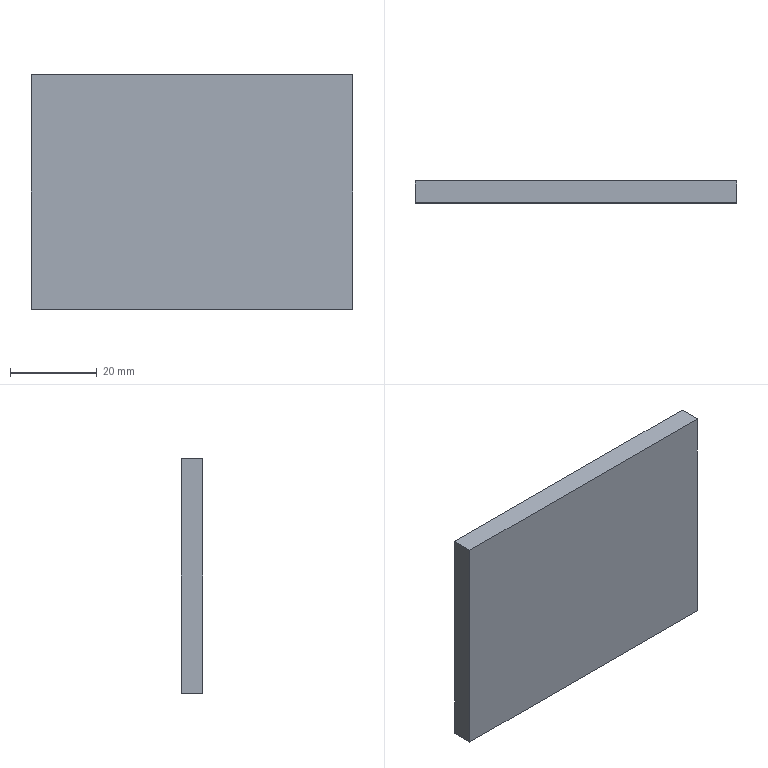Part | STEP file | Guide wheel mechanism revised.sldasm-Part-28 | 1 solid | 6 faces | box 74 x 5 x 54 mm | volume 19980 mm3 | plane 6
STEP:
#1=CARTESIAN_POINT('',(408.,1428.01,502.));
#2=VERTEX_POINT('',#1);
#3=CARTESIAN_POINT('',(408.,1428.01,448.));
#4=VERTEX_POINT('',#3);
#5=CARTESIAN_POINT('',(408.,1428.01,448.));
#6=DIRECTION('',(0.,0.,-1.));
#7=VECTOR('',#6,1000.);
#8=LINE('',#5,#7);
#9=EDGE_CURVE('',#2,#4,#8,.T.);
#10=ORIENTED_EDGE('',*,*,#9,.F.);
#11=CARTESIAN_POINT('',(408.,1433.01,502.));
#12=VERTEX_POINT('',#11);
#13=CARTESIAN_POINT('',(408.,1433.01,502.));
#14=DIRECTION('',(0.,-1.,0.));
#15=VECTOR('',#14,1000.);
#16=LINE('',#13,#15);
#17=EDGE_CURVE('',#12,#2,#16,.T.);
#18=ORIENTED_EDGE('',*,*,#17,.F.);
#19=CARTESIAN_POINT('',(408.,1433.01,448.));
#20=VERTEX_POINT('',#19);
#21=CARTESIAN_POINT('',(408.,1433.01,448.));
#22=DIRECTION('',(0.,0.,-1.));
#23=VECTOR('',#22,1000.);
#24=LINE('',#21,#23);
#25=EDGE_CURVE('',#12,#20,#24,.T.);
#26=ORIENTED_EDGE('',*,*,#25,.T.);
#27=CARTESIAN_POINT('',(408.,1433.01,448.));
#28=DIRECTION('',(0.,-1.,0.));
#29=VECTOR('',#28,1000.);
#30=LINE('',#27,#29);
#31=EDGE_CURVE('',#20,#4,#30,.T.);
#32=ORIENTED_EDGE('',*,*,#31,.T.);
#33=EDGE_LOOP('',(#10,#18,#26,#32));
#34=FACE_OUTER_BOUND('',#33,.T.);
#35=CARTESIAN_POINT('',(408.,1433.01,448.));
#36=DIRECTION('',(-1.,0.,0.));
#37=DIRECTION('',(0.,0.,1.));
#38=AXIS2_PLACEMENT_3D('',#35,#36,#37);
#39=PLANE('',#38);
#40=ADVANCED_FACE('',(#34),#39,.T.);
#41=CARTESIAN_POINT('',(482.,1428.01,502.));
#42=VERTEX_POINT('',#41);
#43=CARTESIAN_POINT('',(408.,1428.01,502.));
#44=DIRECTION('',(-1.,0.,0.));
#45=VECTOR('',#44,1000.);
#46=LINE('',#43,#45);
#47=EDGE_CURVE('',#42,#2,#46,.T.);
#48=ORIENTED_EDGE('',*,*,#47,.F.);
#49=CARTESIAN_POINT('',(482.,1433.01,502.));
#50=VERTEX_POINT('',#49);
#51=CARTESIAN_POINT('',(482.,1433.01,502.));
#52=DIRECTION('',(0.,-1.,0.));
#53=VECTOR('',#52,1000.);
#54=LINE('',#51,#53);
#55=EDGE_CURVE('',#50,#42,#54,.T.);
#56=ORIENTED_EDGE('',*,*,#55,.F.);
#57=CARTESIAN_POINT('',(408.,1433.01,502.));
#58=DIRECTION('',(-1.,0.,0.));
#59=VECTOR('',#58,1000.);
#60=LINE('',#57,#59);
#61=EDGE_CURVE('',#50,#12,#60,.T.);
#62=ORIENTED_EDGE('',*,*,#61,.T.);
#63=ORIENTED_EDGE('',*,*,#17,.T.);
#64=EDGE_LOOP('',(#48,#56,#62,#63));
#65=FACE_OUTER_BOUND('',#64,.T.);
#66=CARTESIAN_POINT('',(408.,1433.01,502.));
#67=DIRECTION('',(0.,0.,1.));
#68=DIRECTION('',(1.,0.,0.));
#69=AXIS2_PLACEMENT_3D('',#66,#67,#68);
#70=PLANE('',#69);
#71=ADVANCED_FACE('',(#65),#70,.T.);
#72=CARTESIAN_POINT('',(482.,1428.01,448.));
#73=VERTEX_POINT('',#72);
#74=CARTESIAN_POINT('',(482.,1428.01,448.));
#75=DIRECTION('',(0.,0.,1.));
#76=VECTOR('',#75,1000.);
#77=LINE('',#74,#76);
#78=EDGE_CURVE('',#73,#42,#77,.T.);
#79=ORIENTED_EDGE('',*,*,#78,.F.);
#80=CARTESIAN_POINT('',(482.,1433.01,448.));
#81=VERTEX_POINT('',#80);
#82=CARTESIAN_POINT('',(482.,1433.01,448.));
#83=DIRECTION('',(0.,-1.,0.));
#84=VECTOR('',#83,1000.);
#85=LINE('',#82,#84);
#86=EDGE_CURVE('',#81,#73,#85,.T.);
#87=ORIENTED_EDGE('',*,*,#86,.F.);
#88=CARTESIAN_POINT('',(482.,1433.01,448.));
#89=DIRECTION('',(0.,0.,1.));
#90=VECTOR('',#89,1000.);
#91=LINE('',#88,#90);
#92=EDGE_CURVE('',#81,#50,#91,.T.);
#93=ORIENTED_EDGE('',*,*,#92,.T.);
#94=ORIENTED_EDGE('',*,*,#55,.T.);
#95=EDGE_LOOP('',(#79,#87,#93,#94));
#96=FACE_OUTER_BOUND('',#95,.T.);
#97=CARTESIAN_POINT('',(482.,1433.01,448.));
#98=DIRECTION('',(1.,0.,0.));
#99=DIRECTION('',(0.,0.,-1.));
#100=AXIS2_PLACEMENT_3D('',#97,#98,#99);
#101=PLANE('',#100);
#102=ADVANCED_FACE('',(#96),#101,.T.);
#103=CARTESIAN_POINT('',(408.,1428.01,448.));
#104=DIRECTION('',(1.,0.,0.));
#105=VECTOR('',#104,1000.);
#106=LINE('',#103,#105);
#107=EDGE_CURVE('',#4,#73,#106,.T.);
#108=ORIENTED_EDGE('',*,*,#107,.F.);
#109=ORIENTED_EDGE('',*,*,#31,.F.);
#110=CARTESIAN_POINT('',(408.,1433.01,448.));
#111=DIRECTION('',(1.,0.,0.));
#112=VECTOR('',#111,1000.);
#113=LINE('',#110,#112);
#114=EDGE_CURVE('',#20,#81,#113,.T.);
#115=ORIENTED_EDGE('',*,*,#114,.T.);
#116=ORIENTED_EDGE('',*,*,#86,.T.);
#117=EDGE_LOOP('',(#108,#109,#115,#116));
#118=FACE_OUTER_BOUND('',#117,.T.);
#119=CARTESIAN_POINT('',(408.,1433.01,448.));
#120=DIRECTION('',(0.,0.,-1.));
#121=DIRECTION('',(-1.,0.,0.));
#122=AXIS2_PLACEMENT_3D('',#119,#120,#121);
#123=PLANE('',#122);
#124=ADVANCED_FACE('',(#118),#123,.T.);
#125=ORIENTED_EDGE('',*,*,#25,.F.);
#126=ORIENTED_EDGE('',*,*,#61,.F.);
#127=ORIENTED_EDGE('',*,*,#92,.F.);
#128=ORIENTED_EDGE('',*,*,#114,.F.);
#129=EDGE_LOOP('',(#125,#126,#127,#128));
#130=FACE_OUTER_BOUND('',#129,.T.);
#131=CARTESIAN_POINT('',(0.,1433.01,0.));
#132=DIRECTION('',(0.,1.,0.));
#133=DIRECTION('',(0.,0.,1.));
#134=AXIS2_PLACEMENT_3D('',#131,#132,#133);
#135=PLANE('',#134);
#136=ADVANCED_FACE('',(#130),#135,.T.);
#137=ORIENTED_EDGE('',*,*,#9,.T.);
#138=ORIENTED_EDGE('',*,*,#107,.T.);
#139=ORIENTED_EDGE('',*,*,#78,.T.);
#140=ORIENTED_EDGE('',*,*,#47,.T.);
#141=EDGE_LOOP('',(#137,#138,#139,#140));
#142=FACE_OUTER_BOUND('',#141,.T.);
#143=CARTESIAN_POINT('',(0.,1428.01,0.));
#144=DIRECTION('',(0.,1.,0.));
#145=DIRECTION('',(0.,0.,1.));
#146=AXIS2_PLACEMENT_3D('',#143,#144,#145);
#147=PLANE('',#146);
#148=ADVANCED_FACE('',(#142),#147,.F.);
#149=CLOSED_SHELL('',(#40,#71,#102,#124,#136,#148));
#150=MANIFOLD_SOLID_BREP('',#149);
#151=CARTESIAN_POINT('',(0.,0.,0.));
#152=DIRECTION('',(0.,0.,1.));
#153=DIRECTION('',(1.,0.,0.));
#154=AXIS2_PLACEMENT_3D('',#151,#152,#153);
#155=(LENGTH_UNIT()NAMED_UNIT(*)SI_UNIT(.MILLI.,.METRE.));
#156=UNCERTAINTY_MEASURE_WITH_UNIT(LENGTH_MEASURE(0.00001),#155,'','');
#157=(NAMED_UNIT(*)PLANE_ANGLE_UNIT()SI_UNIT($,.RADIAN.));
#158=(NAMED_UNIT(*)SI_UNIT($,.STERADIAN.)SOLID_ANGLE_UNIT());
#159=(GEOMETRIC_REPRESENTATION_CONTEXT(3)GLOBAL_UNCERTAINTY_ASSIGNED_CONTEXT((#156))GLOBAL_UNIT_ASSIGNED_CONTEXT((#155,#157,#158))REPRESENTATION_CONTEXT('',''));
#160=ADVANCED_BREP_SHAPE_REPRESENTATION('',(#150,#154),#159);